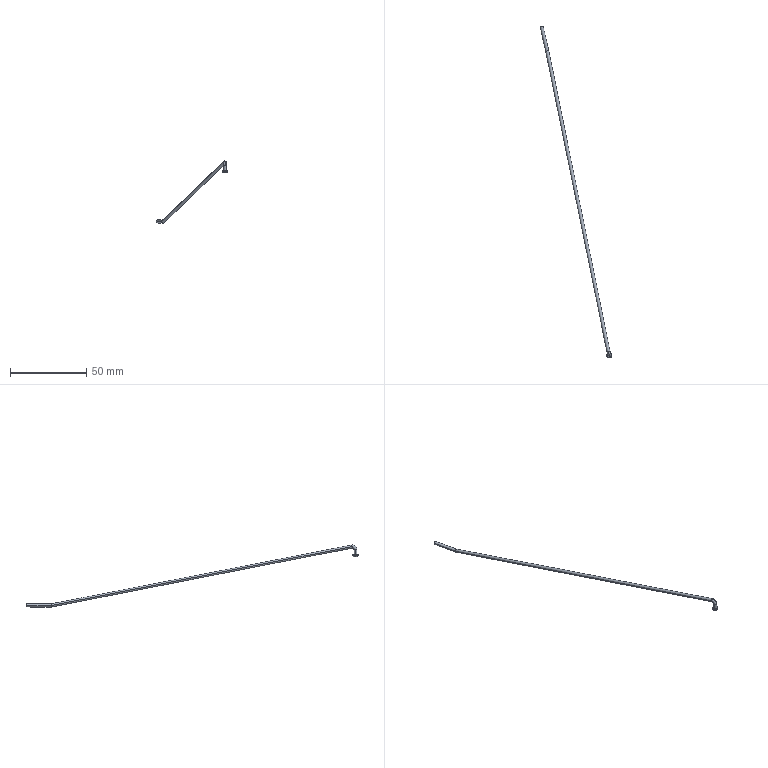Part | STEP file | rear_spoke1 | 1 solid | 15 faces | box 47.236 x 218.366 x 40.79 mm | volume 731.948 mm3 | cylinder 8 | plane 3 | torus 2 | other 2 | commonest cylinder face diameters 2 x6 3.5 x2
STEP:
#1=CARTESIAN_POINT('',(0.,0.,0.));
#2=DIRECTION('',(0.,0.,1.));
#3=DIRECTION('',(1.,0.,0.));
#4=AXIS2_PLACEMENT_3D('',#1,#2,#3);
#5=CARTESIAN_POINT('',(-12.098,26.793,59.29));
#6=VERTEX_POINT('',#5);
#7=CARTESIAN_POINT('',(-10.898,25.813,59.29));
#8=VERTEX_POINT('',#7);
#9=CARTESIAN_POINT('',(-11.098,26.793,59.29));
#10=DIRECTION('',(0.,0.,1.));
#11=DIRECTION('',(1.,0.,0.));
#12=AXIS2_PLACEMENT_3D('',#9,#10,#11);
#13=CIRCLE('',#12,1.);
#14=CARTESIAN_POINT('',(-11.497,28.752,59.29));
#15=DIRECTION('',(-0.9799,-0.1997,0.));
#16=DIRECTION('',(0.1997,-0.9799,0.));
#17=AXIS2_PLACEMENT_3D('',#14,#15,#16);
#18=TOROIDAL_SURFACE('',#17,2.,1.);
#19=CARTESIAN_POINT('',(0.,4.913));
#20=DIRECTION('',(0.,-1.));
#21=VECTOR('',#20,1.);
#22=LINE('',#19,#21);
#23=(GEOMETRIC_REPRESENTATION_CONTEXT(2)PARAMETRIC_REPRESENTATION_CONTEXT()REPRESENTATION_CONTEXT('',''));
#24=DEFINITIONAL_REPRESENTATION('',(#22),#23);
#25=PCURVE('',#18,#24);
#26=CARTESIAN_POINT('',(-11.098,26.793,56.));
#27=DIRECTION('',(0.,0.,1.));
#28=DIRECTION('',(1.,0.,0.));
#29=AXIS2_PLACEMENT_3D('',#26,#27,#28);
#30=CYLINDRICAL_SURFACE('',#29,1.);
#31=CARTESIAN_POINT('',(0.,3.29));
#32=DIRECTION('',(1.,0.));
#33=VECTOR('',#32,1.);
#34=LINE('',#31,#33);
#35=(GEOMETRIC_REPRESENTATION_CONTEXT(2)PARAMETRIC_REPRESENTATION_CONTEXT()REPRESENTATION_CONTEXT('',''));
#36=DEFINITIONAL_REPRESENTATION('',(#34),#35);
#37=PCURVE('',#30,#36);
#38=SURFACE_CURVE('',#13,(#25,#37),.PCURVE_S1.);
#39=EDGE_CURVE('',#6,#8,#38,.T.);
#40=ORIENTED_EDGE('',*,*,#39,.T.);
#41=CARTESIAN_POINT('',(-11.61,29.306,62.236));
#42=VERTEX_POINT('',#41);
#43=CARTESIAN_POINT('',(-11.497,28.752,59.29));
#44=DIRECTION('',(-0.9799,-0.1997,0.));
#45=DIRECTION('',(0.1997,-0.9799,0.));
#46=AXIS2_PLACEMENT_3D('',#43,#44,#45);
#47=CIRCLE('',#46,3.);
#48=CARTESIAN_POINT('',(0.,0.));
#49=DIRECTION('',(1.,0.));
#50=VECTOR('',#49,1.);
#51=LINE('',#48,#50);
#52=(GEOMETRIC_REPRESENTATION_CONTEXT(2)PARAMETRIC_REPRESENTATION_CONTEXT()REPRESENTATION_CONTEXT('',''));
#53=DEFINITIONAL_REPRESENTATION('',(#51),#52);
#54=PCURVE('',#18,#53);
#55=CARTESIAN_POINT('',(-11.497,28.752,59.29));
#56=DIRECTION('',(-0.9799,-0.1997,0.));
#57=DIRECTION('',(0.1997,-0.9799,0.));
#58=AXIS2_PLACEMENT_3D('',#55,#56,#57);
#59=TOROIDAL_SURFACE('',#58,2.,1.);
#60=CARTESIAN_POINT('',(0.,6.283));
#61=CARTESIAN_POINT('',(0.02667,6.283));
#62=CARTESIAN_POINT('',(0.08002,6.283));
#63=CARTESIAN_POINT('',(0.16,6.283));
#64=CARTESIAN_POINT('',(0.2401,6.283));
#65=CARTESIAN_POINT('',(0.3201,6.283));
#66=CARTESIAN_POINT('',(0.4001,6.283));
#67=CARTESIAN_POINT('',(0.4801,6.283));
#68=CARTESIAN_POINT('',(0.5601,6.283));
#69=CARTESIAN_POINT('',(0.6402,6.283));
#70=CARTESIAN_POINT('',(0.7202,6.283));
#71=CARTESIAN_POINT('',(0.8002,6.283));
#72=CARTESIAN_POINT('',(0.8802,6.283));
#73=CARTESIAN_POINT('',(0.9603,6.283));
#74=CARTESIAN_POINT('',(1.04,6.283));
#75=CARTESIAN_POINT('',(1.12,6.283));
#76=CARTESIAN_POINT('',(1.2,6.283));
#77=CARTESIAN_POINT('',(1.28,6.283));
#78=CARTESIAN_POINT('',(1.36,6.283));
#79=CARTESIAN_POINT('',(1.44,6.283));
#80=CARTESIAN_POINT('',(1.52,6.283));
#81=CARTESIAN_POINT('',(1.6,6.283));
#82=CARTESIAN_POINT('',(1.68,6.283));
#83=CARTESIAN_POINT('',(1.734,6.283));
#84=CARTESIAN_POINT('',(1.76,6.283));
#85=B_SPLINE_CURVE_WITH_KNOTS('',3,(#60,#61,#62,#63,#64,#65,#66,#67,#68,#69,#70,#71,#72,#73,#74,#75,#76,#77,#78,#79,#80,#81,#82,#83,#84),.UNSPECIFIED.,.F.,.F.,(4,1,1,1,1,1,1,1,1,1,1,1,1,1,1,1,1,1,1,1,1,1,4),(0.,0.08002,0.16,0.2401,0.3201,0.4001,0.4801,0.5601,0.6402,0.7202,0.8002,0.8802,0.9603,1.04,1.12,1.2,1.28,1.36,1.44,1.52,1.6,1.68,1.76),.QUASI_UNIFORM_KNOTS.);
#86=(GEOMETRIC_REPRESENTATION_CONTEXT(2)PARAMETRIC_REPRESENTATION_CONTEXT()REPRESENTATION_CONTEXT('',''));
#87=DEFINITIONAL_REPRESENTATION('',(#85),#86);
#88=PCURVE('',#59,#87);
#89=SURFACE_CURVE('',#47,(#54,#88),.PCURVE_S1.);
#90=EDGE_CURVE('',#8,#42,#89,.T.);
#91=ORIENTED_EDGE('',*,*,#90,.T.);
#92=CARTESIAN_POINT('',(-12.552,28.922,61.254));
#93=VERTEX_POINT('',#92);
#94=CARTESIAN_POINT('',(-11.573,29.122,61.254));
#95=DIRECTION('',(-0.1961,0.9623,-0.1885));
#96=DIRECTION('',(0.9526,0.2326,0.1961));
#97=AXIS2_PLACEMENT_3D('',#94,#95,#96);
#98=CIRCLE('',#97,1.);
#99=CARTESIAN_POINT('',(1.76,4.913));
#100=DIRECTION('',(0.,-1.));
#101=VECTOR('',#100,1.);
#102=LINE('',#99,#101);
#103=(GEOMETRIC_REPRESENTATION_CONTEXT(2)PARAMETRIC_REPRESENTATION_CONTEXT()REPRESENTATION_CONTEXT('',''));
#104=DEFINITIONAL_REPRESENTATION('',(#102),#103);
#105=PCURVE('',#18,#104);
#106=CARTESIAN_POINT('',(-11.573,29.122,61.254));
#107=DIRECTION('',(-0.1961,0.9623,-0.1885));
#108=DIRECTION('',(-0.9799,-0.1997,0.));
#109=AXIS2_PLACEMENT_3D('',#106,#107,#108);
#110=CYLINDRICAL_SURFACE('',#109,1.);
#111=CARTESIAN_POINT('',(-3.343,0.));
#112=DIRECTION('',(1.,0.));
#113=VECTOR('',#112,1.);
#114=LINE('',#111,#113);
#115=(GEOMETRIC_REPRESENTATION_CONTEXT(2)PARAMETRIC_REPRESENTATION_CONTEXT()REPRESENTATION_CONTEXT('',''));
#116=DEFINITIONAL_REPRESENTATION('',(#114),#115);
#117=PCURVE('',#110,#116);
#118=SURFACE_CURVE('',#98,(#105,#117),.PCURVE_S1.);
#119=EDGE_CURVE('',#93,#42,#118,.T.);
#120=ORIENTED_EDGE('',*,*,#119,.F.);
#121=CARTESIAN_POINT('',(-11.535,28.937,60.272));
#122=VERTEX_POINT('',#121);
#123=CARTESIAN_POINT('',(-11.573,29.122,61.254));
#124=DIRECTION('',(-0.1961,0.9623,-0.1885));
#125=DIRECTION('',(0.9526,0.2326,0.1961));
#126=AXIS2_PLACEMENT_3D('',#123,#124,#125);
#127=CIRCLE('',#126,1.);
#128=CARTESIAN_POINT('',(1.76,4.913));
#129=DIRECTION('',(0.,-1.));
#130=VECTOR('',#129,1.);
#131=LINE('',#128,#130);
#132=(GEOMETRIC_REPRESENTATION_CONTEXT(2)PARAMETRIC_REPRESENTATION_CONTEXT()REPRESENTATION_CONTEXT('',''));
#133=DEFINITIONAL_REPRESENTATION('',(#131),#132);
#134=PCURVE('',#18,#133);
#135=CARTESIAN_POINT('',(-11.573,29.122,61.254));
#136=DIRECTION('',(-0.1961,0.9623,-0.1885));
#137=DIRECTION('',(-0.9799,-0.1997,0.));
#138=AXIS2_PLACEMENT_3D('',#135,#136,#137);
#139=CYLINDRICAL_SURFACE('',#138,1.);
#140=CARTESIAN_POINT('',(2.941,0.));
#141=DIRECTION('',(1.,0.));
#142=VECTOR('',#141,1.);
#143=LINE('',#140,#142);
#144=(GEOMETRIC_REPRESENTATION_CONTEXT(2)PARAMETRIC_REPRESENTATION_CONTEXT()REPRESENTATION_CONTEXT('',''));
#145=DEFINITIONAL_REPRESENTATION('',(#143),#144);
#146=PCURVE('',#139,#145);
#147=SURFACE_CURVE('',#127,(#134,#146),.PCURVE_S1.);
#148=EDGE_CURVE('',#122,#93,#147,.T.);
#149=ORIENTED_EDGE('',*,*,#148,.F.);
#150=CARTESIAN_POINT('',(-11.298,27.772,59.29));
#151=VERTEX_POINT('',#150);
#152=CARTESIAN_POINT('',(-11.497,28.752,59.29));
#153=DIRECTION('',(-0.9799,-0.1997,0.));
#154=DIRECTION('',(0.1997,-0.9799,0.));
#155=AXIS2_PLACEMENT_3D('',#152,#153,#154);
#156=CIRCLE('',#155,1.);
#157=CARTESIAN_POINT('',(0.,3.142));
#158=DIRECTION('',(1.,0.));
#159=VECTOR('',#158,1.);
#160=LINE('',#157,#159);
#161=(GEOMETRIC_REPRESENTATION_CONTEXT(2)PARAMETRIC_REPRESENTATION_CONTEXT()REPRESENTATION_CONTEXT('',''));
#162=DEFINITIONAL_REPRESENTATION('',(#160),#161);
#163=PCURVE('',#18,#162);
#164=CARTESIAN_POINT('',(0.,3.142));
#165=DIRECTION('',(1.,0.));
#166=VECTOR('',#165,1.);
#167=LINE('',#164,#166);
#168=(GEOMETRIC_REPRESENTATION_CONTEXT(2)PARAMETRIC_REPRESENTATION_CONTEXT()REPRESENTATION_CONTEXT('',''));
#169=DEFINITIONAL_REPRESENTATION('',(#167),#168);
#170=PCURVE('',#59,#169);
#171=SURFACE_CURVE('',#156,(#163,#170),.PCURVE_S1.);
#172=EDGE_CURVE('',#151,#122,#171,.T.);
#173=ORIENTED_EDGE('',*,*,#172,.F.);
#174=CARTESIAN_POINT('',(-11.098,26.793,59.29));
#175=DIRECTION('',(0.,0.,1.));
#176=DIRECTION('',(1.,0.,0.));
#177=AXIS2_PLACEMENT_3D('',#174,#175,#176);
#178=CIRCLE('',#177,1.);
#179=CARTESIAN_POINT('',(0.,4.913));
#180=DIRECTION('',(0.,-1.));
#181=VECTOR('',#180,1.);
#182=LINE('',#179,#181);
#183=(GEOMETRIC_REPRESENTATION_CONTEXT(2)PARAMETRIC_REPRESENTATION_CONTEXT()REPRESENTATION_CONTEXT('',''));
#184=DEFINITIONAL_REPRESENTATION('',(#182),#183);
#185=PCURVE('',#18,#184);
#186=CARTESIAN_POINT('',(-11.098,26.793,56.));
#187=DIRECTION('',(0.,0.,1.));
#188=DIRECTION('',(1.,0.,0.));
#189=AXIS2_PLACEMENT_3D('',#186,#187,#188);
#190=CYLINDRICAL_SURFACE('',#189,1.);
#191=CARTESIAN_POINT('',(0.,3.29));
#192=DIRECTION('',(1.,0.));
#193=VECTOR('',#192,1.);
#194=LINE('',#191,#193);
#195=(GEOMETRIC_REPRESENTATION_CONTEXT(2)PARAMETRIC_REPRESENTATION_CONTEXT()REPRESENTATION_CONTEXT('',''));
#196=DEFINITIONAL_REPRESENTATION('',(#194),#195);
#197=PCURVE('',#190,#196);
#198=SURFACE_CURVE('',#178,(#185,#197),.PCURVE_S1.);
#199=EDGE_CURVE('',#151,#6,#198,.T.);
#200=ORIENTED_EDGE('',*,*,#199,.T.);
#201=EDGE_LOOP('',(#40,#91,#120,#149,#173,#200));
#202=FACE_BOUND('',#201,.T.);
#203=ADVANCED_FACE('',(#202),#18,.T.);
#204=CARTESIAN_POINT('',(-9.348,26.793,55.5));
#205=VERTEX_POINT('',#204);
#206=CARTESIAN_POINT('',(-12.848,26.793,55.5));
#207=VERTEX_POINT('',#206);
#208=CARTESIAN_POINT('',(-11.098,26.793,55.5));
#209=DIRECTION('',(0.,0.,1.));
#210=DIRECTION('',(-1.,0.,0.));
#211=AXIS2_PLACEMENT_3D('',#208,#209,#210);
#212=CIRCLE('',#211,1.75);
#213=CARTESIAN_POINT('',(-12.848,26.793,55.5));
#214=CARTESIAN_POINT('',(-12.848,26.793,55.343));
#215=CARTESIAN_POINT('',(-12.817,26.793,55.186));
#216=CARTESIAN_POINT('',(-12.755,26.793,55.037));
#217=CARTESIAN_POINT('',(-12.666,26.793,54.904));
#218=CARTESIAN_POINT('',(-12.444,26.793,54.682));
#219=CARTESIAN_POINT('',(-12.311,26.793,54.593));
#220=CARTESIAN_POINT('',(-12.162,26.793,54.531));
#221=CARTESIAN_POINT('',(-12.005,26.793,54.5));
#222=CARTESIAN_POINT('',(-11.848,26.793,54.5));
#223=B_SPLINE_CURVE_WITH_KNOTS('',5,(#213,#214,#215,#216,#217,#218,#219,#220,#221,#222),.UNSPECIFIED.,.F.,.F.,(6,4,6),(0.,0.7854,1.571),.UNSPECIFIED.);
#224=CARTESIAN_POINT('',(-11.098,26.793,55.5));
#225=DIRECTION('',(0.,0.,-1.));
#226=AXIS1_PLACEMENT('',#224,#225);
#227=SURFACE_OF_REVOLUTION('',#223,#226);
#228=CARTESIAN_POINT('',(6.283,0.));
#229=DIRECTION('',(-1.,0.));
#230=VECTOR('',#229,1.);
#231=LINE('',#228,#230);
#232=(GEOMETRIC_REPRESENTATION_CONTEXT(2)PARAMETRIC_REPRESENTATION_CONTEXT()REPRESENTATION_CONTEXT('',''));
#233=DEFINITIONAL_REPRESENTATION('',(#231),#232);
#234=PCURVE('',#227,#233);
#235=CARTESIAN_POINT('',(-11.098,26.793,54.5));
#236=DIRECTION('',(0.,0.,1.));
#237=DIRECTION('',(1.,0.,0.));
#238=AXIS2_PLACEMENT_3D('',#235,#236,#237);
#239=CYLINDRICAL_SURFACE('',#238,1.75);
#240=CARTESIAN_POINT('',(-3.142,1.));
#241=DIRECTION('',(1.,0.));
#242=VECTOR('',#241,1.);
#243=LINE('',#240,#242);
#244=(GEOMETRIC_REPRESENTATION_CONTEXT(2)PARAMETRIC_REPRESENTATION_CONTEXT()REPRESENTATION_CONTEXT('',''));
#245=DEFINITIONAL_REPRESENTATION('',(#243),#244);
#246=PCURVE('',#239,#245);
#247=SURFACE_CURVE('',#212,(#234,#246),.PCURVE_S1.);
#248=EDGE_CURVE('',#205,#207,#247,.T.);
#249=ORIENTED_EDGE('',*,*,#248,.F.);
#250=CARTESIAN_POINT('',(-10.348,26.793,54.5));
#251=VERTEX_POINT('',#250);
#252=CARTESIAN_POINT('',(-10.348,26.793,55.5));
#253=DIRECTION('',(0.,1.,0.));
#254=DIRECTION('',(-1.,0.,0.));
#255=AXIS2_PLACEMENT_3D('',#252,#253,#254);
#256=CIRCLE('',#255,1.);
#257=CARTESIAN_POINT('',(3.142,-3.142));
#258=DIRECTION('',(0.,1.));
#259=VECTOR('',#258,1.);
#260=LINE('',#257,#259);
#261=(GEOMETRIC_REPRESENTATION_CONTEXT(2)PARAMETRIC_REPRESENTATION_CONTEXT()REPRESENTATION_CONTEXT('',''));
#262=DEFINITIONAL_REPRESENTATION('',(#260),#261);
#263=PCURVE('',#227,#262);
#264=CARTESIAN_POINT('',(-12.848,26.793,55.5));
#265=CARTESIAN_POINT('',(-12.848,26.793,55.343));
#266=CARTESIAN_POINT('',(-12.817,26.793,55.186));
#267=CARTESIAN_POINT('',(-12.755,26.793,55.037));
#268=CARTESIAN_POINT('',(-12.666,26.793,54.904));
#269=CARTESIAN_POINT('',(-12.444,26.793,54.682));
#270=CARTESIAN_POINT('',(-12.311,26.793,54.593));
#271=CARTESIAN_POINT('',(-12.162,26.793,54.531));
#272=CARTESIAN_POINT('',(-12.005,26.793,54.5));
#273=CARTESIAN_POINT('',(-11.848,26.793,54.5));
#274=B_SPLINE_CURVE_WITH_KNOTS('',5,(#264,#265,#266,#267,#268,#269,#270,#271,#272,#273),.UNSPECIFIED.,.F.,.F.,(6,4,6),(0.,0.7854,1.571),.UNSPECIFIED.);
#275=CARTESIAN_POINT('',(-11.098,26.793,55.5));
#276=DIRECTION('',(0.,0.,-1.));
#277=AXIS1_PLACEMENT('',#275,#276);
#278=SURFACE_OF_REVOLUTION('',#274,#277);
#279=CARTESIAN_POINT('',(3.142,-3.142));
#280=DIRECTION('',(0.,1.));
#281=VECTOR('',#280,1.);
#282=LINE('',#279,#281);
#283=(GEOMETRIC_REPRESENTATION_CONTEXT(2)PARAMETRIC_REPRESENTATION_CONTEXT()REPRESENTATION_CONTEXT('',''));
#284=DEFINITIONAL_REPRESENTATION('',(#282),#283);
#285=PCURVE('',#278,#284);
#286=SURFACE_CURVE('',#256,(#263,#285),.PCURVE_S1.);
#287=EDGE_CURVE('',#205,#251,#286,.T.);
#288=ORIENTED_EDGE('',*,*,#287,.T.);
#289=CARTESIAN_POINT('',(-11.848,26.793,54.5));
#290=VERTEX_POINT('',#289);
#291=CARTESIAN_POINT('',(-11.098,26.793,54.5));
#292=DIRECTION('',(0.,0.,-1.));
#293=DIRECTION('',(-1.,0.,0.));
#294=AXIS2_PLACEMENT_3D('',#291,#292,#293);
#295=CIRCLE('',#294,0.75);
#296=CARTESIAN_POINT('',(0.,1.571));
#297=DIRECTION('',(1.,0.));
#298=VECTOR('',#297,1.);
#299=LINE('',#296,#298);
#300=(GEOMETRIC_REPRESENTATION_CONTEXT(2)PARAMETRIC_REPRESENTATION_CONTEXT()REPRESENTATION_CONTEXT('',''));
#301=DEFINITIONAL_REPRESENTATION('',(#299),#300);
#302=PCURVE('',#227,#301);
#303=CARTESIAN_POINT('',(-11.098,26.793,54.5));
#304=DIRECTION('',(0.,0.,-1.));
#305=DIRECTION('',(-1.,0.,0.));
#306=AXIS2_PLACEMENT_3D('',#303,#304,#305);
#307=PLANE('',#306);
#308=CARTESIAN_POINT('',(0.,0.));
#309=DIRECTION('',(1.,0.));
#310=AXIS2_PLACEMENT_2D('',#308,#309);
#311=CIRCLE('',#310,0.75);
#312=(GEOMETRIC_REPRESENTATION_CONTEXT(2)PARAMETRIC_REPRESENTATION_CONTEXT()REPRESENTATION_CONTEXT('',''));
#313=DEFINITIONAL_REPRESENTATION('',(#311),#312);
#314=PCURVE('',#307,#313);
#315=SURFACE_CURVE('',#295,(#302,#314),.PCURVE_S1.);
#316=EDGE_CURVE('',#290,#251,#315,.T.);
#317=ORIENTED_EDGE('',*,*,#316,.F.);
#318=CARTESIAN_POINT('',(-11.848,26.793,55.5));
#319=DIRECTION('',(0.,-1.,0.));
#320=DIRECTION('',(0.,0.,-1.));
#321=AXIS2_PLACEMENT_3D('',#318,#319,#320);
#322=CIRCLE('',#321,1.);
#323=CARTESIAN_POINT('',(0.,-4.712));
#324=DIRECTION('',(0.,1.));
#325=VECTOR('',#324,1.);
#326=LINE('',#323,#325);
#327=(GEOMETRIC_REPRESENTATION_CONTEXT(2)PARAMETRIC_REPRESENTATION_CONTEXT()REPRESENTATION_CONTEXT('',''));
#328=DEFINITIONAL_REPRESENTATION('',(#326),#327);
#329=PCURVE('',#227,#328);
#330=CARTESIAN_POINT('',(6.283,-4.712));
#331=DIRECTION('',(0.,1.));
#332=VECTOR('',#331,1.);
#333=LINE('',#330,#332);
#334=(GEOMETRIC_REPRESENTATION_CONTEXT(2)PARAMETRIC_REPRESENTATION_CONTEXT()REPRESENTATION_CONTEXT('',''));
#335=DEFINITIONAL_REPRESENTATION('',(#333),#334);
#336=PCURVE('',#278,#335);
#337=SURFACE_CURVE('',#322,(#329,#336),.PCURVE_S1.);
#338=EDGE_CURVE('',#207,#290,#337,.T.);
#339=ORIENTED_EDGE('',*,*,#338,.F.);
#340=EDGE_LOOP('',(#249,#288,#317,#339));
#341=FACE_BOUND('',#340,.T.);
#342=ADVANCED_FACE('',(#341),#227,.T.);
#343=ORIENTED_EDGE('',*,*,#248,.T.);
#344=CARTESIAN_POINT('',(-12.848,26.793,56.));
#345=VERTEX_POINT('',#344);
#346=CARTESIAN_POINT('',(-12.848,26.793,54.5));
#347=DIRECTION('',(0.,0.,1.));
#348=VECTOR('',#347,1.);
#349=LINE('',#346,#348);
#350=CARTESIAN_POINT('',(3.142,0.));
#351=DIRECTION('',(0.,1.));
#352=VECTOR('',#351,1.);
#353=LINE('',#350,#352);
#354=(GEOMETRIC_REPRESENTATION_CONTEXT(2)PARAMETRIC_REPRESENTATION_CONTEXT()REPRESENTATION_CONTEXT('',''));
#355=DEFINITIONAL_REPRESENTATION('',(#353),#354);
#356=PCURVE('',#239,#355);
#357=CARTESIAN_POINT('',(-11.098,26.793,54.5));
#358=DIRECTION('',(0.,0.,1.));
#359=DIRECTION('',(1.,0.,0.));
#360=AXIS2_PLACEMENT_3D('',#357,#358,#359);
#361=CYLINDRICAL_SURFACE('',#360,1.75);
#362=CARTESIAN_POINT('',(3.142,0.));
#363=DIRECTION('',(0.,1.));
#364=VECTOR('',#363,1.);
#365=LINE('',#362,#364);
#366=(GEOMETRIC_REPRESENTATION_CONTEXT(2)PARAMETRIC_REPRESENTATION_CONTEXT()REPRESENTATION_CONTEXT('',''));
#367=DEFINITIONAL_REPRESENTATION('',(#365),#366);
#368=PCURVE('',#361,#367);
#369=SURFACE_CURVE('',#349,(#356,#368),.PCURVE_S1.);
#370=EDGE_CURVE('',#207,#345,#369,.T.);
#371=ORIENTED_EDGE('',*,*,#370,.T.);
#372=CARTESIAN_POINT('',(-9.348,26.793,56.));
#373=VERTEX_POINT('',#372);
#374=CARTESIAN_POINT('',(-11.098,26.793,56.));
#375=DIRECTION('',(0.,0.,-1.));
#376=DIRECTION('',(-1.,0.,0.));
#377=AXIS2_PLACEMENT_3D('',#374,#375,#376);
#378=CIRCLE('',#377,1.75);
#379=CARTESIAN_POINT('',(3.142,1.5));
#380=DIRECTION('',(-1.,0.));
#381=VECTOR('',#380,1.);
#382=LINE('',#379,#381);
#383=(GEOMETRIC_REPRESENTATION_CONTEXT(2)PARAMETRIC_REPRESENTATION_CONTEXT()REPRESENTATION_CONTEXT('',''));
#384=DEFINITIONAL_REPRESENTATION('',(#382),#383);
#385=PCURVE('',#239,#384);
#386=CARTESIAN_POINT('',(-11.098,26.793,56.));
#387=DIRECTION('',(0.,0.,-1.));
#388=DIRECTION('',(-1.,0.,0.));
#389=AXIS2_PLACEMENT_3D('',#386,#387,#388);
#390=PLANE('',#389);
#391=CARTESIAN_POINT('',(0.,0.));
#392=DIRECTION('',(1.,0.));
#393=AXIS2_PLACEMENT_2D('',#391,#392);
#394=CIRCLE('',#393,1.75);
#395=(GEOMETRIC_REPRESENTATION_CONTEXT(2)PARAMETRIC_REPRESENTATION_CONTEXT()REPRESENTATION_CONTEXT('',''));
#396=DEFINITIONAL_REPRESENTATION('',(#394),#395);
#397=PCURVE('',#390,#396);
#398=SURFACE_CURVE('',#378,(#385,#397),.PCURVE_S1.);
#399=EDGE_CURVE('',#345,#373,#398,.T.);
#400=ORIENTED_EDGE('',*,*,#399,.T.);
#401=CARTESIAN_POINT('',(-9.348,26.793,54.5));
#402=DIRECTION('',(0.,0.,1.));
#403=VECTOR('',#402,1.);
#404=LINE('',#401,#403);
#405=CARTESIAN_POINT('',(0.,0.));
#406=DIRECTION('',(0.,1.));
#407=VECTOR('',#406,1.);
#408=LINE('',#405,#407);
#409=(GEOMETRIC_REPRESENTATION_CONTEXT(2)PARAMETRIC_REPRESENTATION_CONTEXT()REPRESENTATION_CONTEXT('',''));
#410=DEFINITIONAL_REPRESENTATION('',(#408),#409);
#411=PCURVE('',#239,#410);
#412=CARTESIAN_POINT('',(6.283,0.));
#413=DIRECTION('',(0.,1.));
#414=VECTOR('',#413,1.);
#415=LINE('',#412,#414);
#416=(GEOMETRIC_REPRESENTATION_CONTEXT(2)PARAMETRIC_REPRESENTATION_CONTEXT()REPRESENTATION_CONTEXT('',''));
#417=DEFINITIONAL_REPRESENTATION('',(#415),#416);
#418=PCURVE('',#361,#417);
#419=SURFACE_CURVE('',#404,(#411,#418),.PCURVE_S1.);
#420=EDGE_CURVE('',#205,#373,#419,.T.);
#421=ORIENTED_EDGE('',*,*,#420,.F.);
#422=EDGE_LOOP('',(#343,#371,#400,#421));
#423=FACE_BOUND('',#422,.T.);
#424=ADVANCED_FACE('',(#423),#239,.T.);
#425=ORIENTED_EDGE('',*,*,#119,.T.);
#426=CARTESIAN_POINT('',(-10.593,29.321,61.254));
#427=VERTEX_POINT('',#426);
#428=CARTESIAN_POINT('',(-11.573,29.122,61.254));
#429=DIRECTION('',(-0.1961,0.9623,-0.1885));
#430=DIRECTION('',(0.9526,0.2326,0.1961));
#431=AXIS2_PLACEMENT_3D('',#428,#429,#430);
#432=CIRCLE('',#431,1.);
#433=CARTESIAN_POINT('',(-3.343,0.));
#434=DIRECTION('',(1.,0.));
#435=VECTOR('',#434,1.);
#436=LINE('',#433,#435);
#437=(GEOMETRIC_REPRESENTATION_CONTEXT(2)PARAMETRIC_REPRESENTATION_CONTEXT()REPRESENTATION_CONTEXT('',''));
#438=DEFINITIONAL_REPRESENTATION('',(#436),#437);
#439=PCURVE('',#110,#438);
#440=CARTESIAN_POINT('',(1.76,11.197));
#441=DIRECTION('',(0.,-1.));
#442=VECTOR('',#441,1.);
#443=LINE('',#440,#442);
#444=(GEOMETRIC_REPRESENTATION_CONTEXT(2)PARAMETRIC_REPRESENTATION_CONTEXT()REPRESENTATION_CONTEXT('',''));
#445=DEFINITIONAL_REPRESENTATION('',(#443),#444);
#446=PCURVE('',#59,#445);
#447=SURFACE_CURVE('',#432,(#439,#446),.PCURVE_S1.);
#448=EDGE_CURVE('',#42,#427,#447,.T.);
#449=ORIENTED_EDGE('',*,*,#448,.T.);
#450=CARTESIAN_POINT('',(-50.912,227.13,22.498));
#451=VERTEX_POINT('',#450);
#452=CARTESIAN_POINT('',(-10.593,29.321,61.254));
#453=DIRECTION('',(-0.1961,0.9623,-0.1885));
#454=VECTOR('',#453,1.);
#455=LINE('',#452,#454);
#456=CARTESIAN_POINT('',(3.142,0.));
#457=DIRECTION('',(0.,1.));
#458=VECTOR('',#457,1.);
#459=LINE('',#456,#458);
#460=(GEOMETRIC_REPRESENTATION_CONTEXT(2)PARAMETRIC_REPRESENTATION_CONTEXT()REPRESENTATION_CONTEXT('',''));
#461=DEFINITIONAL_REPRESENTATION('',(#459),#460);
#462=PCURVE('',#110,#461);
#463=CARTESIAN_POINT('',(3.142,0.));
#464=DIRECTION('',(0.,1.));
#465=VECTOR('',#464,1.);
#466=LINE('',#463,#465);
#467=(GEOMETRIC_REPRESENTATION_CONTEXT(2)PARAMETRIC_REPRESENTATION_CONTEXT()REPRESENTATION_CONTEXT('',''));
#468=DEFINITIONAL_REPRESENTATION('',(#466),#467);
#469=PCURVE('',#139,#468);
#470=SURFACE_CURVE('',#455,(#462,#469),.PCURVE_S1.);
#471=EDGE_CURVE('',#427,#451,#470,.T.);
#472=ORIENTED_EDGE('',*,*,#471,.T.);
#473=CARTESIAN_POINT('',(-50.912,227.13,22.5));
#474=VERTEX_POINT('',#473);
#475=CARTESIAN_POINT('',(-50.912,227.13,22.498));
#476=CARTESIAN_POINT('',(-50.912,227.13,22.498));
#477=CARTESIAN_POINT('',(-50.912,227.13,22.499));
#478=CARTESIAN_POINT('',(-50.912,227.13,22.5));
#479=(BOUNDED_CURVE()B_SPLINE_CURVE(3,(#475,#476,#477,#478),.UNSPECIFIED.,.F.,.F.)B_SPLINE_CURVE_WITH_KNOTS((4,4),(1.446,1.448),.PIECEWISE_BEZIER_KNOTS.)CURVE()GEOMETRIC_REPRESENTATION_ITEM()RATIONAL_B_SPLINE_CURVE((1.,1.,1.,1.))REPRESENTATION_ITEM(''));
#480=CARTESIAN_POINT('',(3.142,205.562));
#481=CARTESIAN_POINT('',(3.139,205.562));
#482=B_SPLINE_CURVE_WITH_KNOTS('',1,(#480,#481),.UNSPECIFIED.,.F.,.F.,(2,2),(1.446,1.448),.PIECEWISE_BEZIER_KNOTS.);
#483=(GEOMETRIC_REPRESENTATION_CONTEXT(2)PARAMETRIC_REPRESENTATION_CONTEXT()REPRESENTATION_CONTEXT('',''));
#484=DEFINITIONAL_REPRESENTATION('',(#482),#483);
#485=PCURVE('',#110,#484);
#486=CARTESIAN_POINT('',(-51.818,226.608,22.5));
#487=DIRECTION('',(-0.2229,0.9748,0.));
#488=DIRECTION('',(-0.9748,-0.2229,0.));
#489=AXIS2_PLACEMENT_3D('',#486,#487,#488);
#490=CYLINDRICAL_SURFACE('',#489,1.);
#491=CARTESIAN_POINT('',(3.144,0.3063));
#492=CARTESIAN_POINT('',(3.142,0.3065));
#493=B_SPLINE_CURVE_WITH_KNOTS('',1,(#491,#492),.UNSPECIFIED.,.F.,.F.,(2,2),(1.446,1.448),.PIECEWISE_BEZIER_KNOTS.);
#494=(GEOMETRIC_REPRESENTATION_CONTEXT(2)PARAMETRIC_REPRESENTATION_CONTEXT()REPRESENTATION_CONTEXT('',''));
#495=DEFINITIONAL_REPRESENTATION('',(#493),#494);
#496=PCURVE('',#490,#495);
#497=SURFACE_CURVE('',#479,(#485,#496),.PCURVE_S1.);
#498=EDGE_CURVE('',#451,#474,#497,.T.);
#499=ORIENTED_EDGE('',*,*,#498,.T.);
#500=CARTESIAN_POINT('',(-52.867,226.707,22.502));
#501=VERTEX_POINT('',#500);
#502=CARTESIAN_POINT('',(-50.912,227.13,22.5));
#503=CARTESIAN_POINT('',(-50.954,227.315,24.495));
#504=CARTESIAN_POINT('',(-52.905,226.893,24.498));
#505=CARTESIAN_POINT('',(-52.867,226.707,22.502));
#506=(BOUNDED_CURVE()B_SPLINE_CURVE(3,(#502,#503,#504,#505),.UNSPECIFIED.,.F.,.F.)B_SPLINE_CURVE_WITH_KNOTS((4,4),(1.448,4.587),.PIECEWISE_BEZIER_KNOTS.)CURVE()GEOMETRIC_REPRESENTATION_ITEM()RATIONAL_B_SPLINE_CURVE((1.,0.3341,0.3341,1.))REPRESENTATION_ITEM(''));
#507=CARTESIAN_POINT('',(3.139,205.562));
#508=CARTESIAN_POINT('',(3.109,205.559));
#509=CARTESIAN_POINT('',(3.046,205.553));
#510=CARTESIAN_POINT('',(2.942,205.543));
#511=CARTESIAN_POINT('',(2.828,205.532));
#512=CARTESIAN_POINT('',(2.704,205.52));
#513=CARTESIAN_POINT('',(2.569,205.508));
#514=CARTESIAN_POINT('',(2.424,205.496));
#515=CARTESIAN_POINT('',(2.268,205.485));
#516=CARTESIAN_POINT('',(2.103,205.474));
#517=CARTESIAN_POINT('',(1.93,205.465));
#518=CARTESIAN_POINT('',(1.751,205.458));
#519=CARTESIAN_POINT('',(1.57,205.454));
#520=CARTESIAN_POINT('',(1.388,205.454));
#521=CARTESIAN_POINT('',(1.209,205.456));
#522=CARTESIAN_POINT('',(1.036,205.462));
#523=CARTESIAN_POINT('',(0.8713,205.469));
#524=CARTESIAN_POINT('',(0.7155,205.478));
#525=CARTESIAN_POINT('',(0.5701,205.488));
#526=CARTESIAN_POINT('',(0.4355,205.499));
#527=CARTESIAN_POINT('',(0.3114,205.509));
#528=CARTESIAN_POINT('',(0.1977,205.52));
#529=CARTESIAN_POINT('',(0.09366,205.529));
#530=CARTESIAN_POINT('',(0.0303,205.535));
#531=CARTESIAN_POINT('',(0.,205.538));
#532=B_SPLINE_CURVE_WITH_KNOTS('',3,(#507,#508,#509,#510,#511,#512,#513,#514,#515,#516,#517,#518,#519,#520,#521,#522,#523,#524,#525,#526,#527,#528,#529,#530,#531),.UNSPECIFIED.,.F.,.F.,(4,1,1,1,1,1,1,1,1,1,1,1,1,1,1,1,1,1,1,1,1,1,4),(1.448,1.591,1.733,1.876,2.019,2.161,2.304,2.447,2.589,2.732,2.875,3.017,3.16,3.303,3.446,3.588,3.731,3.874,4.016,4.159,4.302,4.444,4.587),.QUASI_UNIFORM_KNOTS.);
#533=(GEOMETRIC_REPRESENTATION_CONTEXT(2)PARAMETRIC_REPRESENTATION_CONTEXT()REPRESENTATION_CONTEXT('',''));
#534=DEFINITIONAL_REPRESENTATION('',(#532),#533);
#535=PCURVE('',#110,#534);
#536=CARTESIAN_POINT('',(-51.818,226.608,22.5));
#537=DIRECTION('',(-0.2229,0.9748,0.));
#538=DIRECTION('',(-0.9748,-0.2229,0.));
#539=AXIS2_PLACEMENT_3D('',#536,#537,#538);
#540=CYLINDRICAL_SURFACE('',#539,1.);
#541=CARTESIAN_POINT('',(3.142,0.3065));
#542=CARTESIAN_POINT('',(3.111,0.3094));
#543=CARTESIAN_POINT('',(3.048,0.3155));
#544=CARTESIAN_POINT('',(2.944,0.3254));
#545=CARTESIAN_POINT('',(2.83,0.3363));
#546=CARTESIAN_POINT('',(2.706,0.3478));
#547=CARTESIAN_POINT('',(2.571,0.3599));
#548=CARTESIAN_POINT('',(2.426,0.372));
#549=CARTESIAN_POINT('',(2.27,0.3838));
#550=CARTESIAN_POINT('',(2.105,0.3945));
#551=CARTESIAN_POINT('',(1.932,0.4035));
#552=CARTESIAN_POINT('',(1.754,0.4102));
#553=CARTESIAN_POINT('',(1.572,0.4139));
#554=CARTESIAN_POINT('',(1.39,0.4145));
#555=CARTESIAN_POINT('',(1.212,0.412));
#556=CARTESIAN_POINT('',(1.039,0.4066));
#557=CARTESIAN_POINT('',(0.8735,0.3991));
#558=CARTESIAN_POINT('',(0.7178,0.39));
#559=CARTESIAN_POINT('',(0.5724,0.3799));
#560=CARTESIAN_POINT('',(0.4377,0.3694));
#561=CARTESIAN_POINT('',(0.3137,0.3589));
#562=CARTESIAN_POINT('',(0.2,0.3488));
#563=CARTESIAN_POINT('',(0.09592,0.3391));
#564=CARTESIAN_POINT('',(0.03256,0.3331));
#565=CARTESIAN_POINT('',(0.002257,0.3302));
#566=B_SPLINE_CURVE_WITH_KNOTS('',3,(#541,#542,#543,#544,#545,#546,#547,#548,#549,#550,#551,#552,#553,#554,#555,#556,#557,#558,#559,#560,#561,#562,#563,#564,#565),.UNSPECIFIED.,.F.,.F.,(4,1,1,1,1,1,1,1,1,1,1,1,1,1,1,1,1,1,1,1,1,1,4),(1.448,1.591,1.733,1.876,2.019,2.161,2.304,2.447,2.589,2.732,2.875,3.017,3.16,3.303,3.446,3.588,3.731,3.874,4.016,4.159,4.302,4.444,4.587),.QUASI_UNIFORM_KNOTS.);
#567=(GEOMETRIC_REPRESENTATION_CONTEXT(2)PARAMETRIC_REPRESENTATION_CONTEXT()REPRESENTATION_CONTEXT('',''));
#568=DEFINITIONAL_REPRESENTATION('',(#566),#567);
#569=PCURVE('',#540,#568);
#570=SURFACE_CURVE('',#506,(#535,#569),.PCURVE_S1.);
#571=EDGE_CURVE('',#474,#501,#570,.T.);
#572=ORIENTED_EDGE('',*,*,#571,.T.);
#573=CARTESIAN_POINT('',(-12.552,28.922,61.254));
#574=DIRECTION('',(-0.1961,0.9623,-0.1885));
#575=VECTOR('',#574,1.);
#576=LINE('',#573,#575);
#577=CARTESIAN_POINT('',(0.,0.));
#578=DIRECTION('',(0.,1.));
#579=VECTOR('',#578,1.);
#580=LINE('',#577,#579);
#581=(GEOMETRIC_REPRESENTATION_CONTEXT(2)PARAMETRIC_REPRESENTATION_CONTEXT()REPRESENTATION_CONTEXT('',''));
#582=DEFINITIONAL_REPRESENTATION('',(#580),#581);
#583=PCURVE('',#110,#582);
#584=CARTESIAN_POINT('',(6.283,0.));
#585=DIRECTION('',(0.,1.));
#586=VECTOR('',#585,1.);
#587=LINE('',#584,#586);
#588=(GEOMETRIC_REPRESENTATION_CONTEXT(2)PARAMETRIC_REPRESENTATION_CONTEXT()REPRESENTATION_CONTEXT('',''));
#589=DEFINITIONAL_REPRESENTATION('',(#587),#588);
#590=PCURVE('',#139,#589);
#591=SURFACE_CURVE('',#576,(#583,#590),.PCURVE_S1.);
#592=EDGE_CURVE('',#93,#501,#591,.T.);
#593=ORIENTED_EDGE('',*,*,#592,.F.);
#594=EDGE_LOOP('',(#425,#449,#472,#499,#572,#593));
#595=FACE_BOUND('',#594,.T.);
#596=ADVANCED_FACE('',(#595),#110,.T.);
#597=CARTESIAN_POINT('',(-10.098,26.793,56.));
#598=VERTEX_POINT('',#597);
#599=CARTESIAN_POINT('',(-12.098,26.793,56.));
#600=VERTEX_POINT('',#599);
#601=CARTESIAN_POINT('',(-11.098,26.793,56.));
#602=DIRECTION('',(0.,0.,1.));
#603=DIRECTION('',(1.,0.,0.));
#604=AXIS2_PLACEMENT_3D('',#601,#602,#603);
#605=CIRCLE('',#604,1.);
#606=CARTESIAN_POINT('',(0.,0.));
#607=DIRECTION('',(1.,0.));
#608=VECTOR('',#607,1.);
#609=LINE('',#606,#608);
#610=(GEOMETRIC_REPRESENTATION_CONTEXT(2)PARAMETRIC_REPRESENTATION_CONTEXT()REPRESENTATION_CONTEXT('',''));
#611=DEFINITIONAL_REPRESENTATION('',(#609),#610);
#612=PCURVE('',#190,#611);
#613=CARTESIAN_POINT('',(-1.,0.));
#614=CARTESIAN_POINT('',(-1.,1.732));
#615=CARTESIAN_POINT('',(0.5,0.866));
#616=CARTESIAN_POINT('',(2.,0.));
#617=CARTESIAN_POINT('',(0.5,-0.866));
#618=CARTESIAN_POINT('',(-1.,-1.732));
#619=CARTESIAN_POINT('',(-1.,0.));
#620=(BOUNDED_CURVE()B_SPLINE_CURVE(2,(#613,#614,#615,#616,#617,#618,#619),.UNSPECIFIED.,.T.,.F.)B_SPLINE_CURVE_WITH_KNOTS((1,2,2,2,2,1),(-2.094,0.,2.094,4.189,6.283,8.378),.UNSPECIFIED.)CURVE()GEOMETRIC_REPRESENTATION_ITEM()RATIONAL_B_SPLINE_CURVE((1.,0.5,1.,0.5,1.,0.5,1.))REPRESENTATION_ITEM(''));
#621=(GEOMETRIC_REPRESENTATION_CONTEXT(2)PARAMETRIC_REPRESENTATION_CONTEXT()REPRESENTATION_CONTEXT('',''));
#622=DEFINITIONAL_REPRESENTATION('',(#620),#621);
#623=PCURVE('',#390,#622);
#624=SURFACE_CURVE('',#605,(#612,#623),.PCURVE_S1.);
#625=EDGE_CURVE('',#598,#600,#624,.T.);
#626=ORIENTED_EDGE('',*,*,#625,.T.);
#627=CARTESIAN_POINT('',(-12.098,26.793,56.));
#628=DIRECTION('',(0.,0.,1.));
#629=VECTOR('',#628,1.);
#630=LINE('',#627,#629);
#631=CARTESIAN_POINT('',(3.142,0.));
#632=DIRECTION('',(0.,1.));
#633=VECTOR('',#632,1.);
#634=LINE('',#631,#633);
#635=(GEOMETRIC_REPRESENTATION_CONTEXT(2)PARAMETRIC_REPRESENTATION_CONTEXT()REPRESENTATION_CONTEXT('',''));
#636=DEFINITIONAL_REPRESENTATION('',(#634),#635);
#637=PCURVE('',#190,#636);
#638=CARTESIAN_POINT('',(3.142,0.));
#639=DIRECTION('',(0.,1.));
#640=VECTOR('',#639,1.);
#641=LINE('',#638,#640);
#642=(GEOMETRIC_REPRESENTATION_CONTEXT(2)PARAMETRIC_REPRESENTATION_CONTEXT()REPRESENTATION_CONTEXT('',''));
#643=DEFINITIONAL_REPRESENTATION('',(#641),#642);
#644=PCURVE('',#30,#643);
#645=SURFACE_CURVE('',#630,(#637,#644),.PCURVE_S1.);
#646=EDGE_CURVE('',#600,#6,#645,.T.);
#647=ORIENTED_EDGE('',*,*,#646,.T.);
#648=ORIENTED_EDGE('',*,*,#199,.F.);
#649=CARTESIAN_POINT('',(-10.098,26.793,59.29));
#650=VERTEX_POINT('',#649);
#651=CARTESIAN_POINT('',(-11.098,26.793,59.29));
#652=DIRECTION('',(0.,0.,1.));
#653=DIRECTION('',(1.,0.,0.));
#654=AXIS2_PLACEMENT_3D('',#651,#652,#653);
#655=CIRCLE('',#654,1.);
#656=CARTESIAN_POINT('',(0.,3.29));
#657=DIRECTION('',(1.,0.));
#658=VECTOR('',#657,1.);
#659=LINE('',#656,#658);
#660=(GEOMETRIC_REPRESENTATION_CONTEXT(2)PARAMETRIC_REPRESENTATION_CONTEXT()REPRESENTATION_CONTEXT('',''));
#661=DEFINITIONAL_REPRESENTATION('',(#659),#660);
#662=PCURVE('',#190,#661);
#663=CARTESIAN_POINT('',(0.,4.913));
#664=DIRECTION('',(0.,-1.));
#665=VECTOR('',#664,1.);
#666=LINE('',#663,#665);
#667=(GEOMETRIC_REPRESENTATION_CONTEXT(2)PARAMETRIC_REPRESENTATION_CONTEXT()REPRESENTATION_CONTEXT('',''));
#668=DEFINITIONAL_REPRESENTATION('',(#666),#667);
#669=PCURVE('',#59,#668);
#670=SURFACE_CURVE('',#655,(#662,#669),.PCURVE_S1.);
#671=EDGE_CURVE('',#650,#151,#670,.T.);
#672=ORIENTED_EDGE('',*,*,#671,.F.);
#673=CARTESIAN_POINT('',(-10.098,26.793,56.));
#674=DIRECTION('',(0.,0.,1.));
#675=VECTOR('',#674,1.);
#676=LINE('',#673,#675);
#677=CARTESIAN_POINT('',(0.,0.));
#678=DIRECTION('',(0.,1.));
#679=VECTOR('',#678,1.);
#680=LINE('',#677,#679);
#681=(GEOMETRIC_REPRESENTATION_CONTEXT(2)PARAMETRIC_REPRESENTATION_CONTEXT()REPRESENTATION_CONTEXT('',''));
#682=DEFINITIONAL_REPRESENTATION('',(#680),#681);
#683=PCURVE('',#190,#682);
#684=CARTESIAN_POINT('',(6.283,0.));
#685=DIRECTION('',(0.,1.));
#686=VECTOR('',#685,1.);
#687=LINE('',#684,#686);
#688=(GEOMETRIC_REPRESENTATION_CONTEXT(2)PARAMETRIC_REPRESENTATION_CONTEXT()REPRESENTATION_CONTEXT('',''));
#689=DEFINITIONAL_REPRESENTATION('',(#687),#688);
#690=PCURVE('',#30,#689);
#691=SURFACE_CURVE('',#676,(#683,#690),.PCURVE_S1.);
#692=EDGE_CURVE('',#598,#650,#691,.T.);
#693=ORIENTED_EDGE('',*,*,#692,.F.);
#694=EDGE_LOOP('',(#626,#647,#648,#672,#693));
#695=FACE_BOUND('',#694,.T.);
#696=ADVANCED_FACE('',(#695),#190,.T.);
#697=ORIENTED_EDGE('',*,*,#571,.F.);
#698=CARTESIAN_POINT('',(-54.634,243.408,22.5));
#699=VERTEX_POINT('',#698);
#700=CARTESIAN_POINT('',(-50.844,226.831,22.5));
#701=DIRECTION('',(-0.2229,0.9748,0.));
#702=VECTOR('',#701,1.);
#703=LINE('',#700,#702);
#704=CARTESIAN_POINT('',(3.142,0.));
#705=DIRECTION('',(0.,1.));
#706=VECTOR('',#705,1.);
#707=LINE('',#704,#706);
#708=(GEOMETRIC_REPRESENTATION_CONTEXT(2)PARAMETRIC_REPRESENTATION_CONTEXT()REPRESENTATION_CONTEXT('',''));
#709=DEFINITIONAL_REPRESENTATION('',(#707),#708);
#710=PCURVE('',#540,#709);
#711=CARTESIAN_POINT('',(3.142,0.));
#712=DIRECTION('',(0.,1.));
#713=VECTOR('',#712,1.);
#714=LINE('',#711,#713);
#715=(GEOMETRIC_REPRESENTATION_CONTEXT(2)PARAMETRIC_REPRESENTATION_CONTEXT()REPRESENTATION_CONTEXT('',''));
#716=DEFINITIONAL_REPRESENTATION('',(#714),#715);
#717=PCURVE('',#490,#716);
#718=SURFACE_CURVE('',#703,(#710,#717),.PCURVE_S1.);
#719=EDGE_CURVE('',#474,#699,#718,.T.);
#720=ORIENTED_EDGE('',*,*,#719,.T.);
#721=CARTESIAN_POINT('',(-56.584,242.962,22.5));
#722=VERTEX_POINT('',#721);
#723=CARTESIAN_POINT('',(-55.609,243.185,22.5));
#724=DIRECTION('',(-0.2229,0.9748,0.));
#725=DIRECTION('',(0.9556,0.2185,0.1975));
#726=AXIS2_PLACEMENT_3D('',#723,#724,#725);
#727=CIRCLE('',#726,1.);
#728=CARTESIAN_POINT('',(-3.34,17.005));
#729=DIRECTION('',(1.,0.));
#730=VECTOR('',#729,1.);
#731=LINE('',#728,#730);
#732=(GEOMETRIC_REPRESENTATION_CONTEXT(2)PARAMETRIC_REPRESENTATION_CONTEXT()REPRESENTATION_CONTEXT('',''));
#733=DEFINITIONAL_REPRESENTATION('',(#731),#732);
#734=PCURVE('',#540,#733);
#735=CARTESIAN_POINT('',(-55.609,243.185,22.5));
#736=DIRECTION('',(-0.2229,0.9748,0.));
#737=DIRECTION('',(0.9556,0.2185,0.1975));
#738=AXIS2_PLACEMENT_3D('',#735,#736,#737);
#739=PLANE('',#738);
#740=CARTESIAN_POINT('',(0.,0.));
#741=DIRECTION('',(1.,0.));
#742=AXIS2_PLACEMENT_2D('',#740,#741);
#743=CIRCLE('',#742,1.);
#744=(GEOMETRIC_REPRESENTATION_CONTEXT(2)PARAMETRIC_REPRESENTATION_CONTEXT()REPRESENTATION_CONTEXT('',''));
#745=DEFINITIONAL_REPRESENTATION('',(#743),#744);
#746=PCURVE('',#739,#745);
#747=SURFACE_CURVE('',#727,(#734,#746),.PCURVE_S1.);
#748=EDGE_CURVE('',#722,#699,#747,.T.);
#749=ORIENTED_EDGE('',*,*,#748,.F.);
#750=CARTESIAN_POINT('',(-52.867,226.707,22.5));
#751=VERTEX_POINT('',#750);
#752=CARTESIAN_POINT('',(-52.793,226.385,22.5));
#753=DIRECTION('',(-0.2229,0.9748,0.));
#754=VECTOR('',#753,1.);
#755=LINE('',#752,#754);
#756=CARTESIAN_POINT('',(0.,0.));
#757=DIRECTION('',(0.,1.));
#758=VECTOR('',#757,1.);
#759=LINE('',#756,#758);
#760=(GEOMETRIC_REPRESENTATION_CONTEXT(2)PARAMETRIC_REPRESENTATION_CONTEXT()REPRESENTATION_CONTEXT('',''));
#761=DEFINITIONAL_REPRESENTATION('',(#759),#760);
#762=PCURVE('',#540,#761);
#763=CARTESIAN_POINT('',(6.283,0.));
#764=DIRECTION('',(0.,1.));
#765=VECTOR('',#764,1.);
#766=LINE('',#763,#765);
#767=(GEOMETRIC_REPRESENTATION_CONTEXT(2)PARAMETRIC_REPRESENTATION_CONTEXT()REPRESENTATION_CONTEXT('',''));
#768=DEFINITIONAL_REPRESENTATION('',(#766),#767);
#769=PCURVE('',#490,#768);
#770=SURFACE_CURVE('',#755,(#762,#769),.PCURVE_S1.);
#771=EDGE_CURVE('',#751,#722,#770,.T.);
#772=ORIENTED_EDGE('',*,*,#771,.F.);
#773=CARTESIAN_POINT('',(-52.867,226.707,22.502));
#774=CARTESIAN_POINT('',(-52.867,226.707,22.502));
#775=CARTESIAN_POINT('',(-52.867,226.707,22.501));
#776=CARTESIAN_POINT('',(-52.867,226.707,22.5));
#777=(BOUNDED_CURVE()B_SPLINE_CURVE(3,(#773,#774,#775,#776),.UNSPECIFIED.,.F.,.F.)B_SPLINE_CURVE_WITH_KNOTS((4,4),(4.587,4.589),.PIECEWISE_BEZIER_KNOTS.)CURVE()GEOMETRIC_REPRESENTATION_ITEM()RATIONAL_B_SPLINE_CURVE((1.,1.,1.,1.))REPRESENTATION_ITEM(''));
#778=CARTESIAN_POINT('',(0.002257,0.3302));
#779=CARTESIAN_POINT('',(0.,0.33));
#780=B_SPLINE_CURVE_WITH_KNOTS('',1,(#778,#779),.UNSPECIFIED.,.F.,.F.,(2,2),(4.587,4.589),.PIECEWISE_BEZIER_KNOTS.);
#781=(GEOMETRIC_REPRESENTATION_CONTEXT(2)PARAMETRIC_REPRESENTATION_CONTEXT()REPRESENTATION_CONTEXT('',''));
#782=DEFINITIONAL_REPRESENTATION('',(#780),#781);
#783=PCURVE('',#540,#782);
#784=CARTESIAN_POINT('',(6.283,205.538));
#785=CARTESIAN_POINT('',(6.281,205.538));
#786=B_SPLINE_CURVE_WITH_KNOTS('',1,(#784,#785),.UNSPECIFIED.,.F.,.F.,(2,2),(4.587,4.589),.PIECEWISE_BEZIER_KNOTS.);
#787=(GEOMETRIC_REPRESENTATION_CONTEXT(2)PARAMETRIC_REPRESENTATION_CONTEXT()REPRESENTATION_CONTEXT('',''));
#788=DEFINITIONAL_REPRESENTATION('',(#786),#787);
#789=PCURVE('',#139,#788);
#790=SURFACE_CURVE('',#777,(#783,#789),.PCURVE_S1.);
#791=EDGE_CURVE('',#501,#751,#790,.T.);
#792=ORIENTED_EDGE('',*,*,#791,.F.);
#793=EDGE_LOOP('',(#697,#720,#749,#772,#792));
#794=FACE_BOUND('',#793,.T.);
#795=ADVANCED_FACE('',(#794),#540,.T.);
#796=ORIENTED_EDGE('',*,*,#471,.F.);
#797=CARTESIAN_POINT('',(-11.573,29.122,61.254));
#798=DIRECTION('',(-0.1961,0.9623,-0.1885));
#799=DIRECTION('',(0.9526,0.2326,0.1961));
#800=AXIS2_PLACEMENT_3D('',#797,#798,#799);
#801=CIRCLE('',#800,1.);
#802=CARTESIAN_POINT('',(2.941,0.));
#803=DIRECTION('',(1.,0.));
#804=VECTOR('',#803,1.);
#805=LINE('',#802,#804);
#806=(GEOMETRIC_REPRESENTATION_CONTEXT(2)PARAMETRIC_REPRESENTATION_CONTEXT()REPRESENTATION_CONTEXT('',''));
#807=DEFINITIONAL_REPRESENTATION('',(#805),#806);
#808=PCURVE('',#139,#807);
#809=CARTESIAN_POINT('',(1.76,4.913));
#810=DIRECTION('',(0.,-1.));
#811=VECTOR('',#810,1.);
#812=LINE('',#809,#811);
#813=(GEOMETRIC_REPRESENTATION_CONTEXT(2)PARAMETRIC_REPRESENTATION_CONTEXT()REPRESENTATION_CONTEXT('',''));
#814=DEFINITIONAL_REPRESENTATION('',(#812),#813);
#815=PCURVE('',#59,#814);
#816=SURFACE_CURVE('',#801,(#808,#815),.PCURVE_S1.);
#817=EDGE_CURVE('',#427,#122,#816,.T.);
#818=ORIENTED_EDGE('',*,*,#817,.T.);
#819=ORIENTED_EDGE('',*,*,#148,.T.);
#820=ORIENTED_EDGE('',*,*,#592,.T.);
#821=ORIENTED_EDGE('',*,*,#791,.T.);
#822=CARTESIAN_POINT('',(-52.867,226.707,22.5));
#823=CARTESIAN_POINT('',(-52.824,226.522,20.505));
#824=CARTESIAN_POINT('',(-50.874,226.943,20.502));
#825=CARTESIAN_POINT('',(-50.912,227.13,22.498));
#826=(BOUNDED_CURVE()B_SPLINE_CURVE(3,(#822,#823,#824,#825),.UNSPECIFIED.,.F.,.F.)B_SPLINE_CURVE_WITH_KNOTS((4,4),(4.589,7.729),.PIECEWISE_BEZIER_KNOTS.)CURVE()GEOMETRIC_REPRESENTATION_ITEM()RATIONAL_B_SPLINE_CURVE((1.,0.3341,0.3341,1.))REPRESENTATION_ITEM(''));
#827=CARTESIAN_POINT('',(6.281,205.538));
#828=CARTESIAN_POINT('',(6.251,205.541));
#829=CARTESIAN_POINT('',(6.187,205.547));
#830=CARTESIAN_POINT('',(6.083,205.557));
#831=CARTESIAN_POINT('',(5.969,205.568));
#832=CARTESIAN_POINT('',(5.845,205.58));
#833=CARTESIAN_POINT('',(5.711,205.592));
#834=CARTESIAN_POINT('',(5.565,205.604));
#835=CARTESIAN_POINT('',(5.41,205.616));
#836=CARTESIAN_POINT('',(5.244,205.626));
#837=CARTESIAN_POINT('',(5.072,205.635));
#838=CARTESIAN_POINT('',(4.893,205.642));
#839=CARTESIAN_POINT('',(4.711,205.646));
#840=CARTESIAN_POINT('',(4.53,205.646));
#841=CARTESIAN_POINT('',(4.351,205.644));
#842=CARTESIAN_POINT('',(4.178,205.638));
#843=CARTESIAN_POINT('',(4.013,205.631));
#844=CARTESIAN_POINT('',(3.857,205.622));
#845=CARTESIAN_POINT('',(3.712,205.612));
#846=CARTESIAN_POINT('',(3.577,205.601));
#847=CARTESIAN_POINT('',(3.453,205.591));
#848=CARTESIAN_POINT('',(3.339,205.581));
#849=CARTESIAN_POINT('',(3.235,205.571));
#850=CARTESIAN_POINT('',(3.172,205.565));
#851=CARTESIAN_POINT('',(3.142,205.562));
#852=B_SPLINE_CURVE_WITH_KNOTS('',3,(#827,#828,#829,#830,#831,#832,#833,#834,#835,#836,#837,#838,#839,#840,#841,#842,#843,#844,#845,#846,#847,#848,#849,#850,#851),.UNSPECIFIED.,.F.,.F.,(4,1,1,1,1,1,1,1,1,1,1,1,1,1,1,1,1,1,1,1,1,1,4),(4.589,4.732,4.875,5.018,5.16,5.303,5.446,5.588,5.731,5.874,6.016,6.159,6.302,6.444,6.587,6.73,6.873,7.015,7.158,7.301,7.443,7.586,7.729),.QUASI_UNIFORM_KNOTS.);
#853=(GEOMETRIC_REPRESENTATION_CONTEXT(2)PARAMETRIC_REPRESENTATION_CONTEXT()REPRESENTATION_CONTEXT('',''));
#854=DEFINITIONAL_REPRESENTATION('',(#852),#853);
#855=PCURVE('',#139,#854);
#856=CARTESIAN_POINT('',(6.283,0.33));
#857=CARTESIAN_POINT('',(6.253,0.3272));
#858=CARTESIAN_POINT('',(6.19,0.3211));
#859=CARTESIAN_POINT('',(6.085,0.3111));
#860=CARTESIAN_POINT('',(5.972,0.3003));
#861=CARTESIAN_POINT('',(5.848,0.2887));
#862=CARTESIAN_POINT('',(5.713,0.2767));
#863=CARTESIAN_POINT('',(5.568,0.2645));
#864=CARTESIAN_POINT('',(5.412,0.2528));
#865=CARTESIAN_POINT('',(5.247,0.242));
#866=CARTESIAN_POINT('',(5.074,0.233));
#867=CARTESIAN_POINT('',(4.895,0.2264));
#868=CARTESIAN_POINT('',(4.714,0.2226));
#869=CARTESIAN_POINT('',(4.532,0.2221));
#870=CARTESIAN_POINT('',(4.353,0.2246));
#871=CARTESIAN_POINT('',(4.18,0.2299));
#872=CARTESIAN_POINT('',(4.015,0.2374));
#873=CARTESIAN_POINT('',(3.859,0.2466));
#874=CARTESIAN_POINT('',(3.714,0.2567));
#875=CARTESIAN_POINT('',(3.579,0.2672));
#876=CARTESIAN_POINT('',(3.455,0.2776));
#877=CARTESIAN_POINT('',(3.342,0.2878));
#878=CARTESIAN_POINT('',(3.238,0.2974));
#879=CARTESIAN_POINT('',(3.174,0.3034));
#880=CARTESIAN_POINT('',(3.144,0.3063));
#881=B_SPLINE_CURVE_WITH_KNOTS('',3,(#856,#857,#858,#859,#860,#861,#862,#863,#864,#865,#866,#867,#868,#869,#870,#871,#872,#873,#874,#875,#876,#877,#878,#879,#880),.UNSPECIFIED.,.F.,.F.,(4,1,1,1,1,1,1,1,1,1,1,1,1,1,1,1,1,1,1,1,1,1,4),(4.589,4.732,4.875,5.018,5.16,5.303,5.446,5.588,5.731,5.874,6.016,6.159,6.302,6.444,6.587,6.73,6.873,7.015,7.158,7.301,7.443,7.586,7.729),.QUASI_UNIFORM_KNOTS.);
#882=(GEOMETRIC_REPRESENTATION_CONTEXT(2)PARAMETRIC_REPRESENTATION_CONTEXT()REPRESENTATION_CONTEXT('',''));
#883=DEFINITIONAL_REPRESENTATION('',(#881),#882);
#884=PCURVE('',#490,#883);
#885=SURFACE_CURVE('',#826,(#855,#884),.PCURVE_S1.);
#886=EDGE_CURVE('',#751,#451,#885,.T.);
#887=ORIENTED_EDGE('',*,*,#886,.T.);
#888=EDGE_LOOP('',(#796,#818,#819,#820,#821,#887));
#889=FACE_BOUND('',#888,.T.);
#890=ADVANCED_FACE('',(#889),#139,.T.);
#891=ORIENTED_EDGE('',*,*,#90,.F.);
#892=CARTESIAN_POINT('',(-11.098,26.793,59.29));
#893=DIRECTION('',(0.,0.,1.));
#894=DIRECTION('',(1.,0.,0.));
#895=AXIS2_PLACEMENT_3D('',#892,#893,#894);
#896=CIRCLE('',#895,1.);
#897=CARTESIAN_POINT('',(0.,11.197));
#898=DIRECTION('',(0.,-1.));
#899=VECTOR('',#898,1.);
#900=LINE('',#897,#899);
#901=(GEOMETRIC_REPRESENTATION_CONTEXT(2)PARAMETRIC_REPRESENTATION_CONTEXT()REPRESENTATION_CONTEXT('',''));
#902=DEFINITIONAL_REPRESENTATION('',(#900),#901);
#903=PCURVE('',#59,#902);
#904=CARTESIAN_POINT('',(0.,3.29));
#905=DIRECTION('',(1.,0.));
#906=VECTOR('',#905,1.);
#907=LINE('',#904,#906);
#908=(GEOMETRIC_REPRESENTATION_CONTEXT(2)PARAMETRIC_REPRESENTATION_CONTEXT()REPRESENTATION_CONTEXT('',''));
#909=DEFINITIONAL_REPRESENTATION('',(#907),#908);
#910=PCURVE('',#30,#909);
#911=SURFACE_CURVE('',#896,(#903,#910),.PCURVE_S1.);
#912=EDGE_CURVE('',#8,#650,#911,.T.);
#913=ORIENTED_EDGE('',*,*,#912,.T.);
#914=ORIENTED_EDGE('',*,*,#671,.T.);
#915=ORIENTED_EDGE('',*,*,#172,.T.);
#916=ORIENTED_EDGE('',*,*,#817,.F.);
#917=ORIENTED_EDGE('',*,*,#448,.F.);
#918=EDGE_LOOP('',(#891,#913,#914,#915,#916,#917));
#919=FACE_BOUND('',#918,.T.);
#920=ADVANCED_FACE('',(#919),#59,.T.);
#921=ORIENTED_EDGE('',*,*,#646,.F.);
#922=CARTESIAN_POINT('',(-11.098,26.793,56.));
#923=DIRECTION('',(0.,0.,1.));
#924=DIRECTION('',(1.,0.,0.));
#925=AXIS2_PLACEMENT_3D('',#922,#923,#924);
#926=CIRCLE('',#925,1.);
#927=CARTESIAN_POINT('',(0.,0.));
#928=DIRECTION('',(1.,0.));
#929=VECTOR('',#928,1.);
#930=LINE('',#927,#929);
#931=(GEOMETRIC_REPRESENTATION_CONTEXT(2)PARAMETRIC_REPRESENTATION_CONTEXT()REPRESENTATION_CONTEXT('',''));
#932=DEFINITIONAL_REPRESENTATION('',(#930),#931);
#933=PCURVE('',#30,#932);
#934=CARTESIAN_POINT('',(-1.,0.));
#935=CARTESIAN_POINT('',(-1.,1.732));
#936=CARTESIAN_POINT('',(0.5,0.866));
#937=CARTESIAN_POINT('',(2.,0.));
#938=CARTESIAN_POINT('',(0.5,-0.866));
#939=CARTESIAN_POINT('',(-1.,-1.732));
#940=CARTESIAN_POINT('',(-1.,0.));
#941=(BOUNDED_CURVE()B_SPLINE_CURVE(2,(#934,#935,#936,#937,#938,#939,#940),.UNSPECIFIED.,.T.,.F.)B_SPLINE_CURVE_WITH_KNOTS((1,2,2,2,2,1),(-2.094,0.,2.094,4.189,6.283,8.378),.UNSPECIFIED.)CURVE()GEOMETRIC_REPRESENTATION_ITEM()RATIONAL_B_SPLINE_CURVE((1.,0.5,1.,0.5,1.,0.5,1.))REPRESENTATION_ITEM(''));
#942=(GEOMETRIC_REPRESENTATION_CONTEXT(2)PARAMETRIC_REPRESENTATION_CONTEXT()REPRESENTATION_CONTEXT('',''));
#943=DEFINITIONAL_REPRESENTATION('',(#941),#942);
#944=PCURVE('',#390,#943);
#945=SURFACE_CURVE('',#926,(#933,#944),.PCURVE_S1.);
#946=EDGE_CURVE('',#600,#598,#945,.T.);
#947=ORIENTED_EDGE('',*,*,#946,.T.);
#948=ORIENTED_EDGE('',*,*,#692,.T.);
#949=ORIENTED_EDGE('',*,*,#912,.F.);
#950=ORIENTED_EDGE('',*,*,#39,.F.);
#951=EDGE_LOOP('',(#921,#947,#948,#949,#950));
#952=FACE_BOUND('',#951,.T.);
#953=ADVANCED_FACE('',(#952),#30,.T.);
#954=ORIENTED_EDGE('',*,*,#719,.F.);
#955=ORIENTED_EDGE('',*,*,#498,.F.);
#956=ORIENTED_EDGE('',*,*,#886,.F.);
#957=ORIENTED_EDGE('',*,*,#771,.T.);
#958=CARTESIAN_POINT('',(-55.609,243.185,22.5));
#959=DIRECTION('',(-0.2229,0.9748,0.));
#960=DIRECTION('',(0.9556,0.2185,0.1975));
#961=AXIS2_PLACEMENT_3D('',#958,#959,#960);
#962=CIRCLE('',#961,1.);
#963=CARTESIAN_POINT('',(2.943,17.005));
#964=DIRECTION('',(1.,0.));
#965=VECTOR('',#964,1.);
#966=LINE('',#963,#965);
#967=(GEOMETRIC_REPRESENTATION_CONTEXT(2)PARAMETRIC_REPRESENTATION_CONTEXT()REPRESENTATION_CONTEXT('',''));
#968=DEFINITIONAL_REPRESENTATION('',(#966),#967);
#969=PCURVE('',#490,#968);
#970=CARTESIAN_POINT('',(0.,0.));
#971=DIRECTION('',(1.,0.));
#972=AXIS2_PLACEMENT_2D('',#970,#971);
#973=CIRCLE('',#972,1.);
#974=(GEOMETRIC_REPRESENTATION_CONTEXT(2)PARAMETRIC_REPRESENTATION_CONTEXT()REPRESENTATION_CONTEXT('',''));
#975=DEFINITIONAL_REPRESENTATION('',(#973),#974);
#976=PCURVE('',#739,#975);
#977=SURFACE_CURVE('',#962,(#969,#976),.PCURVE_S1.);
#978=EDGE_CURVE('',#699,#722,#977,.T.);
#979=ORIENTED_EDGE('',*,*,#978,.F.);
#980=EDGE_LOOP('',(#954,#955,#956,#957,#979));
#981=FACE_BOUND('',#980,.T.);
#982=ADVANCED_FACE('',(#981),#490,.T.);
#983=ORIENTED_EDGE('',*,*,#748,.T.);
#984=ORIENTED_EDGE('',*,*,#978,.T.);
#985=EDGE_LOOP('',(#983,#984));
#986=FACE_BOUND('',#985,.T.);
#987=ADVANCED_FACE('',(#986),#739,.T.);
#988=ORIENTED_EDGE('',*,*,#370,.F.);
#989=CARTESIAN_POINT('',(-11.098,26.793,55.5));
#990=DIRECTION('',(0.,0.,1.));
#991=DIRECTION('',(-1.,0.,0.));
#992=AXIS2_PLACEMENT_3D('',#989,#990,#991);
#993=CIRCLE('',#992,1.75);
#994=CARTESIAN_POINT('',(3.142,1.));
#995=DIRECTION('',(1.,0.));
#996=VECTOR('',#995,1.);
#997=LINE('',#994,#996);
#998=(GEOMETRIC_REPRESENTATION_CONTEXT(2)PARAMETRIC_REPRESENTATION_CONTEXT()REPRESENTATION_CONTEXT('',''));
#999=DEFINITIONAL_REPRESENTATION('',(#997),#998);
#1000=PCURVE('',#361,#999);
#1001=CARTESIAN_POINT('',(6.283,0.));
#1002=DIRECTION('',(-1.,0.));
#1003=VECTOR('',#1002,1.);
#1004=LINE('',#1001,#1003);
#1005=(GEOMETRIC_REPRESENTATION_CONTEXT(2)PARAMETRIC_REPRESENTATION_CONTEXT()REPRESENTATION_CONTEXT('',''));
#1006=DEFINITIONAL_REPRESENTATION('',(#1004),#1005);
#1007=PCURVE('',#278,#1006);
#1008=SURFACE_CURVE('',#993,(#1000,#1007),.PCURVE_S1.);
#1009=EDGE_CURVE('',#207,#205,#1008,.T.);
#1010=ORIENTED_EDGE('',*,*,#1009,.T.);
#1011=ORIENTED_EDGE('',*,*,#420,.T.);
#1012=CARTESIAN_POINT('',(-11.098,26.793,56.));
#1013=DIRECTION('',(0.,0.,-1.));
#1014=DIRECTION('',(-1.,0.,0.));
#1015=AXIS2_PLACEMENT_3D('',#1012,#1013,#1014);
#1016=CIRCLE('',#1015,1.75);
#1017=CARTESIAN_POINT('',(9.425,1.5));
#1018=DIRECTION('',(-1.,0.));
#1019=VECTOR('',#1018,1.);
#1020=LINE('',#1017,#1019);
#1021=(GEOMETRIC_REPRESENTATION_CONTEXT(2)PARAMETRIC_REPRESENTATION_CONTEXT()REPRESENTATION_CONTEXT('',''));
#1022=DEFINITIONAL_REPRESENTATION('',(#1020),#1021);
#1023=PCURVE('',#361,#1022);
#1024=CARTESIAN_POINT('',(0.,0.));
#1025=DIRECTION('',(1.,0.));
#1026=AXIS2_PLACEMENT_2D('',#1024,#1025);
#1027=CIRCLE('',#1026,1.75);
#1028=(GEOMETRIC_REPRESENTATION_CONTEXT(2)PARAMETRIC_REPRESENTATION_CONTEXT()REPRESENTATION_CONTEXT('',''));
#1029=DEFINITIONAL_REPRESENTATION('',(#1027),#1028);
#1030=PCURVE('',#390,#1029);
#1031=SURFACE_CURVE('',#1016,(#1023,#1030),.PCURVE_S1.);
#1032=EDGE_CURVE('',#373,#345,#1031,.T.);
#1033=ORIENTED_EDGE('',*,*,#1032,.T.);
#1034=EDGE_LOOP('',(#988,#1010,#1011,#1033));
#1035=FACE_BOUND('',#1034,.T.);
#1036=ADVANCED_FACE('',(#1035),#361,.T.);
#1037=ORIENTED_EDGE('',*,*,#316,.T.);
#1038=CARTESIAN_POINT('',(-11.098,26.793,54.5));
#1039=DIRECTION('',(0.,0.,-1.));
#1040=DIRECTION('',(-1.,0.,0.));
#1041=AXIS2_PLACEMENT_3D('',#1038,#1039,#1040);
#1042=CIRCLE('',#1041,0.75);
#1043=CARTESIAN_POINT('',(0.,0.));
#1044=DIRECTION('',(1.,0.));
#1045=AXIS2_PLACEMENT_2D('',#1043,#1044);
#1046=CIRCLE('',#1045,0.75);
#1047=(GEOMETRIC_REPRESENTATION_CONTEXT(2)PARAMETRIC_REPRESENTATION_CONTEXT()REPRESENTATION_CONTEXT('',''));
#1048=DEFINITIONAL_REPRESENTATION('',(#1046),#1047);
#1049=PCURVE('',#307,#1048);
#1050=CARTESIAN_POINT('',(0.,1.571));
#1051=DIRECTION('',(1.,0.));
#1052=VECTOR('',#1051,1.);
#1053=LINE('',#1050,#1052);
#1054=(GEOMETRIC_REPRESENTATION_CONTEXT(2)PARAMETRIC_REPRESENTATION_CONTEXT()REPRESENTATION_CONTEXT('',''));
#1055=DEFINITIONAL_REPRESENTATION('',(#1053),#1054);
#1056=PCURVE('',#278,#1055);
#1057=SURFACE_CURVE('',#1042,(#1049,#1056),.PCURVE_S1.);
#1058=EDGE_CURVE('',#251,#290,#1057,.T.);
#1059=ORIENTED_EDGE('',*,*,#1058,.T.);
#1060=EDGE_LOOP('',(#1037,#1059));
#1061=FACE_BOUND('',#1060,.T.);
#1062=ADVANCED_FACE('',(#1061),#307,.T.);
#1063=ORIENTED_EDGE('',*,*,#625,.F.);
#1064=ORIENTED_EDGE('',*,*,#946,.F.);
#1065=EDGE_LOOP('',(#1063,#1064));
#1066=FACE_BOUND('',#1065,.T.);
#1067=ORIENTED_EDGE('',*,*,#1032,.F.);
#1068=ORIENTED_EDGE('',*,*,#399,.F.);
#1069=EDGE_LOOP('',(#1067,#1068));
#1070=FACE_BOUND('',#1069,.T.);
#1071=ADVANCED_FACE('',(#1066,#1070),#390,.F.);
#1072=ORIENTED_EDGE('',*,*,#287,.F.);
#1073=ORIENTED_EDGE('',*,*,#1009,.F.);
#1074=ORIENTED_EDGE('',*,*,#338,.T.);
#1075=ORIENTED_EDGE('',*,*,#1058,.F.);
#1076=EDGE_LOOP('',(#1072,#1073,#1074,#1075));
#1077=FACE_BOUND('',#1076,.T.);
#1078=ADVANCED_FACE('',(#1077),#278,.T.);
#1079=CLOSED_SHELL('',(#203,#342,#424,#596,#696,#795,#890,#920,#953,#982,#987,#1036,#1062,#1071,#1078));
#1080=MANIFOLD_SOLID_BREP('',#1079);
#1081=(LENGTH_UNIT()NAMED_UNIT(*)SI_UNIT(.MILLI.,.METRE.));
#1082=UNCERTAINTY_MEASURE_WITH_UNIT(LENGTH_MEASURE(0.0000001),#1081,'','');
#1083=(NAMED_UNIT(*)PLANE_ANGLE_UNIT()SI_UNIT($,.RADIAN.));
#1084=(NAMED_UNIT(*)SI_UNIT($,.STERADIAN.)SOLID_ANGLE_UNIT());
#1085=(GEOMETRIC_REPRESENTATION_CONTEXT(3)GLOBAL_UNCERTAINTY_ASSIGNED_CONTEXT((#1082))GLOBAL_UNIT_ASSIGNED_CONTEXT((#1081,#1083,#1084))REPRESENTATION_CONTEXT('',''));
#1086=ADVANCED_BREP_SHAPE_REPRESENTATION('',(#4,#1080),#1085);